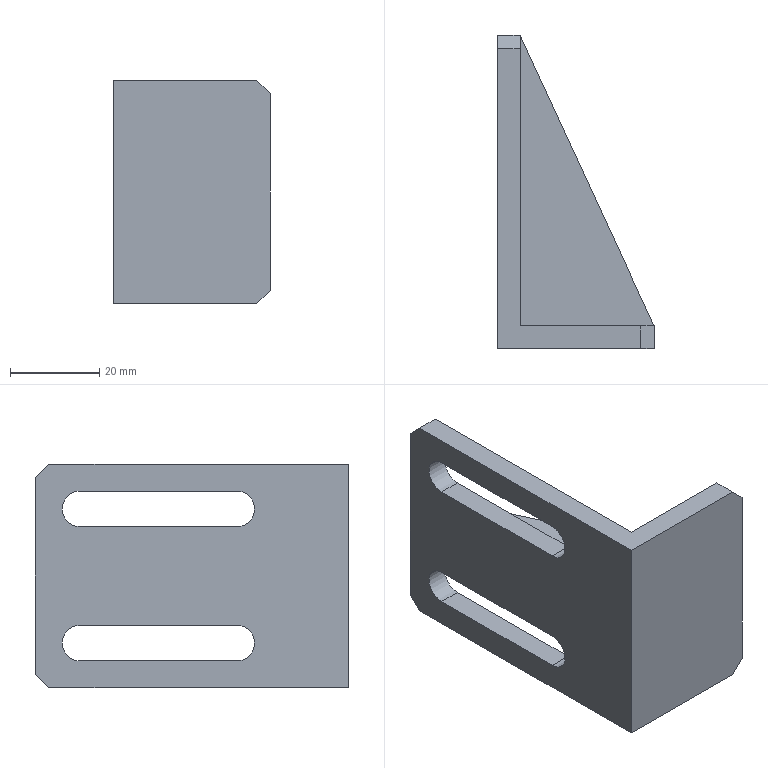Part | STEP file | Guide wheel mechanism revised.sldasm-Part-62 | 1 solid | 25 faces | box 35 x 70 x 50 mm | volume 26482 mm3 | plane 21 | cylinder 4 | commonest cylinder face diameters 8 x4
STEP:
#1=CARTESIAN_POINT('',(35.,5.,-2.5));
#2=VERTEX_POINT('',#1);
#3=CARTESIAN_POINT('',(35.,5.,-22.));
#4=VERTEX_POINT('',#3);
#5=CARTESIAN_POINT('',(35.,5.,25.));
#6=DIRECTION('',(0.,0.,-1.));
#7=VECTOR('',#6,1000.);
#8=LINE('',#5,#7);
#9=EDGE_CURVE('',#2,#4,#8,.T.);
#10=ORIENTED_EDGE('',*,*,#9,.T.);
#11=CARTESIAN_POINT('',(32.,5.,-25.));
#12=VERTEX_POINT('',#11);
#13=CARTESIAN_POINT('',(41.,5.,-16.));
#14=DIRECTION('',(-0.7071,0.,-0.7071));
#15=VECTOR('',#14,1000.);
#16=LINE('',#13,#15);
#17=EDGE_CURVE('',#4,#12,#16,.T.);
#18=ORIENTED_EDGE('',*,*,#17,.T.);
#19=CARTESIAN_POINT('',(5.,5.,-25.));
#20=VERTEX_POINT('',#19);
#21=CARTESIAN_POINT('',(0.,5.,-25.));
#22=DIRECTION('',(1.,0.,0.));
#23=VECTOR('',#22,1000.);
#24=LINE('',#21,#23);
#25=EDGE_CURVE('',#20,#12,#24,.T.);
#26=ORIENTED_EDGE('',*,*,#25,.F.);
#27=CARTESIAN_POINT('',(5.,5.,-2.5));
#28=VERTEX_POINT('',#27);
#29=CARTESIAN_POINT('',(5.,5.,25.));
#30=DIRECTION('',(0.,0.,-1.));
#31=VECTOR('',#30,1000.);
#32=LINE('',#29,#31);
#33=EDGE_CURVE('',#28,#20,#32,.T.);
#34=ORIENTED_EDGE('',*,*,#33,.F.);
#35=CARTESIAN_POINT('',(35.,5.,-2.5));
#36=DIRECTION('',(1.,0.,0.));
#37=VECTOR('',#36,1000.);
#38=LINE('',#35,#37);
#39=EDGE_CURVE('',#28,#2,#38,.T.);
#40=ORIENTED_EDGE('',*,*,#39,.T.);
#41=EDGE_LOOP('',(#10,#18,#26,#34,#40));
#42=FACE_OUTER_BOUND('',#41,.T.);
#43=CARTESIAN_POINT('',(0.,5.,25.));
#44=DIRECTION('',(0.,1.,0.));
#45=DIRECTION('',(0.,0.,1.));
#46=AXIS2_PLACEMENT_3D('',#43,#44,#45);
#47=PLANE('',#46);
#48=ADVANCED_FACE('',(#42),#47,.T.);
#49=CARTESIAN_POINT('',(5.,60.,-19.));
#50=VERTEX_POINT('',#49);
#51=CARTESIAN_POINT('',(5.,60.,-11.));
#52=VERTEX_POINT('',#51);
#53=CARTESIAN_POINT('',(5.,60.,-15.));
#54=DIRECTION('',(1.,0.,0.));
#55=DIRECTION('',(0.,0.,-1.));
#56=AXIS2_PLACEMENT_3D('',#53,#54,#55);
#57=CIRCLE('',#56,4.);
#58=EDGE_CURVE('',#50,#52,#57,.T.);
#59=ORIENTED_EDGE('',*,*,#58,.F.);
#60=CARTESIAN_POINT('',(5.,25.,-19.));
#61=VERTEX_POINT('',#60);
#62=CARTESIAN_POINT('',(5.,60.,-19.));
#63=DIRECTION('',(0.,1.,0.));
#64=VECTOR('',#63,1000.);
#65=LINE('',#62,#64);
#66=EDGE_CURVE('',#61,#50,#65,.T.);
#67=ORIENTED_EDGE('',*,*,#66,.F.);
#68=CARTESIAN_POINT('',(5.,25.,-11.));
#69=VERTEX_POINT('',#68);
#70=CARTESIAN_POINT('',(5.,25.,-15.));
#71=DIRECTION('',(1.,0.,0.));
#72=DIRECTION('',(0.,0.,-1.));
#73=AXIS2_PLACEMENT_3D('',#70,#71,#72);
#74=CIRCLE('',#73,4.);
#75=EDGE_CURVE('',#69,#61,#74,.T.);
#76=ORIENTED_EDGE('',*,*,#75,.F.);
#77=CARTESIAN_POINT('',(5.,60.,-11.));
#78=DIRECTION('',(0.,-1.,0.));
#79=VECTOR('',#78,1000.);
#80=LINE('',#77,#79);
#81=EDGE_CURVE('',#52,#69,#80,.T.);
#82=ORIENTED_EDGE('',*,*,#81,.F.);
#83=EDGE_LOOP('',(#59,#67,#76,#82));
#84=FACE_BOUND('',#83,.T.);
#85=CARTESIAN_POINT('',(5.,67.,-25.));
#86=VERTEX_POINT('',#85);
#87=CARTESIAN_POINT('',(5.,0.,-25.));
#88=DIRECTION('',(0.,-1.,0.));
#89=VECTOR('',#88,1000.);
#90=LINE('',#87,#89);
#91=EDGE_CURVE('',#86,#20,#90,.T.);
#92=ORIENTED_EDGE('',*,*,#91,.F.);
#93=CARTESIAN_POINT('',(5.,70.,-22.));
#94=VERTEX_POINT('',#93);
#95=CARTESIAN_POINT('',(5.,58.5,-33.5));
#96=DIRECTION('',(0.,0.7071,0.7071));
#97=VECTOR('',#96,1000.);
#98=LINE('',#95,#97);
#99=EDGE_CURVE('',#86,#94,#98,.T.);
#100=ORIENTED_EDGE('',*,*,#99,.T.);
#101=CARTESIAN_POINT('',(5.,70.,-2.5));
#102=VERTEX_POINT('',#101);
#103=CARTESIAN_POINT('',(5.,70.,25.));
#104=DIRECTION('',(0.,0.,-1.));
#105=VECTOR('',#104,1000.);
#106=LINE('',#103,#105);
#107=EDGE_CURVE('',#102,#94,#106,.T.);
#108=ORIENTED_EDGE('',*,*,#107,.F.);
#109=CARTESIAN_POINT('',(5.,5.,-2.5));
#110=DIRECTION('',(0.,-1.,0.));
#111=VECTOR('',#110,1000.);
#112=LINE('',#109,#111);
#113=EDGE_CURVE('',#102,#28,#112,.T.);
#114=ORIENTED_EDGE('',*,*,#113,.T.);
#115=ORIENTED_EDGE('',*,*,#33,.T.);
#116=EDGE_LOOP('',(#92,#100,#108,#114,#115));
#117=FACE_OUTER_BOUND('',#116,.T.);
#118=CARTESIAN_POINT('',(5.,0.,25.));
#119=DIRECTION('',(1.,0.,0.));
#120=DIRECTION('',(0.,0.,-1.));
#121=AXIS2_PLACEMENT_3D('',#118,#119,#120);
#122=PLANE('',#121);
#123=ADVANCED_FACE('',(#84,#117),#122,.T.);
#124=CARTESIAN_POINT('',(35.,0.,22.));
#125=VERTEX_POINT('',#124);
#126=CARTESIAN_POINT('',(35.,0.,-22.));
#127=VERTEX_POINT('',#126);
#128=CARTESIAN_POINT('',(35.,0.,25.));
#129=DIRECTION('',(0.,0.,-1.));
#130=VECTOR('',#129,1000.);
#131=LINE('',#128,#130);
#132=EDGE_CURVE('',#125,#127,#131,.T.);
#133=ORIENTED_EDGE('',*,*,#132,.F.);
#134=CARTESIAN_POINT('',(32.,0.,25.));
#135=VERTEX_POINT('',#134);
#136=CARTESIAN_POINT('',(35.,0.,22.));
#137=DIRECTION('',(-0.7071,0.,0.7071));
#138=VECTOR('',#137,1000.);
#139=LINE('',#136,#138);
#140=EDGE_CURVE('',#125,#135,#139,.T.);
#141=ORIENTED_EDGE('',*,*,#140,.T.);
#142=CARTESIAN_POINT('',(0.,0.,25.));
#143=VERTEX_POINT('',#142);
#144=CARTESIAN_POINT('',(0.,0.,25.));
#145=DIRECTION('',(1.,0.,0.));
#146=VECTOR('',#145,1000.);
#147=LINE('',#144,#146);
#148=EDGE_CURVE('',#143,#135,#147,.T.);
#149=ORIENTED_EDGE('',*,*,#148,.F.);
#150=CARTESIAN_POINT('',(0.,0.,-25.));
#151=VERTEX_POINT('',#150);
#152=CARTESIAN_POINT('',(0.,0.,25.));
#153=DIRECTION('',(0.,0.,-1.));
#154=VECTOR('',#153,1000.);
#155=LINE('',#152,#154);
#156=EDGE_CURVE('',#143,#151,#155,.T.);
#157=ORIENTED_EDGE('',*,*,#156,.T.);
#158=CARTESIAN_POINT('',(32.,0.,-25.));
#159=VERTEX_POINT('',#158);
#160=CARTESIAN_POINT('',(0.,0.,-25.));
#161=DIRECTION('',(1.,0.,0.));
#162=VECTOR('',#161,1000.);
#163=LINE('',#160,#162);
#164=EDGE_CURVE('',#151,#159,#163,.T.);
#165=ORIENTED_EDGE('',*,*,#164,.T.);
#166=CARTESIAN_POINT('',(32.,0.,-25.));
#167=DIRECTION('',(0.7071,0.,0.7071));
#168=VECTOR('',#167,1000.);
#169=LINE('',#166,#168);
#170=EDGE_CURVE('',#159,#127,#169,.T.);
#171=ORIENTED_EDGE('',*,*,#170,.T.);
#172=EDGE_LOOP('',(#133,#141,#149,#157,#165,#171));
#173=FACE_OUTER_BOUND('',#172,.T.);
#174=CARTESIAN_POINT('',(0.,0.,25.));
#175=DIRECTION('',(0.,1.,0.));
#176=DIRECTION('',(0.,0.,1.));
#177=AXIS2_PLACEMENT_3D('',#174,#175,#176);
#178=PLANE('',#177);
#179=ADVANCED_FACE('',(#173),#178,.F.);
#180=CARTESIAN_POINT('',(35.,5.,22.));
#181=VERTEX_POINT('',#180);
#182=CARTESIAN_POINT('',(35.,5.,2.5));
#183=VERTEX_POINT('',#182);
#184=CARTESIAN_POINT('',(35.,5.,25.));
#185=DIRECTION('',(0.,0.,-1.));
#186=VECTOR('',#185,1000.);
#187=LINE('',#184,#186);
#188=EDGE_CURVE('',#181,#183,#187,.T.);
#189=ORIENTED_EDGE('',*,*,#188,.F.);
#190=CARTESIAN_POINT('',(35.,0.,22.));
#191=DIRECTION('',(0.,-1.,0.));
#192=VECTOR('',#191,1000.);
#193=LINE('',#190,#192);
#194=EDGE_CURVE('',#181,#125,#193,.T.);
#195=ORIENTED_EDGE('',*,*,#194,.T.);
#196=ORIENTED_EDGE('',*,*,#132,.T.);
#197=CARTESIAN_POINT('',(35.,5.,-22.));
#198=DIRECTION('',(0.,1.,0.));
#199=VECTOR('',#198,1000.);
#200=LINE('',#197,#199);
#201=EDGE_CURVE('',#127,#4,#200,.T.);
#202=ORIENTED_EDGE('',*,*,#201,.T.);
#203=ORIENTED_EDGE('',*,*,#9,.F.);
#204=CARTESIAN_POINT('',(35.,5.,2.5));
#205=DIRECTION('',(0.,0.,-1.));
#206=VECTOR('',#205,1000.);
#207=LINE('',#204,#206);
#208=EDGE_CURVE('',#183,#2,#207,.T.);
#209=ORIENTED_EDGE('',*,*,#208,.F.);
#210=EDGE_LOOP('',(#189,#195,#196,#202,#203,#209));
#211=FACE_OUTER_BOUND('',#210,.T.);
#212=CARTESIAN_POINT('',(35.,5.,25.));
#213=DIRECTION('',(1.,0.,0.));
#214=DIRECTION('',(0.,0.,-1.));
#215=AXIS2_PLACEMENT_3D('',#212,#213,#214);
#216=PLANE('',#215);
#217=ADVANCED_FACE('',(#211),#216,.T.);
#218=CARTESIAN_POINT('',(5.,5.,25.));
#219=VERTEX_POINT('',#218);
#220=CARTESIAN_POINT('',(32.,5.,25.));
#221=VERTEX_POINT('',#220);
#222=CARTESIAN_POINT('',(0.,5.,25.));
#223=DIRECTION('',(1.,0.,0.));
#224=VECTOR('',#223,1000.);
#225=LINE('',#222,#224);
#226=EDGE_CURVE('',#219,#221,#225,.T.);
#227=ORIENTED_EDGE('',*,*,#226,.T.);
#228=CARTESIAN_POINT('',(16.,5.,41.));
#229=DIRECTION('',(0.7071,0.,-0.7071));
#230=VECTOR('',#229,1000.);
#231=LINE('',#228,#230);
#232=EDGE_CURVE('',#221,#181,#231,.T.);
#233=ORIENTED_EDGE('',*,*,#232,.T.);
#234=ORIENTED_EDGE('',*,*,#188,.T.);
#235=CARTESIAN_POINT('',(5.,5.,2.5));
#236=VERTEX_POINT('',#235);
#237=CARTESIAN_POINT('',(35.,5.,2.5));
#238=DIRECTION('',(1.,0.,0.));
#239=VECTOR('',#238,1000.);
#240=LINE('',#237,#239);
#241=EDGE_CURVE('',#236,#183,#240,.T.);
#242=ORIENTED_EDGE('',*,*,#241,.F.);
#243=CARTESIAN_POINT('',(5.,5.,25.));
#244=DIRECTION('',(0.,0.,-1.));
#245=VECTOR('',#244,1000.);
#246=LINE('',#243,#245);
#247=EDGE_CURVE('',#219,#236,#246,.T.);
#248=ORIENTED_EDGE('',*,*,#247,.F.);
#249=EDGE_LOOP('',(#227,#233,#234,#242,#248));
#250=FACE_OUTER_BOUND('',#249,.T.);
#251=CARTESIAN_POINT('',(0.,5.,25.));
#252=DIRECTION('',(0.,1.,0.));
#253=DIRECTION('',(0.,0.,1.));
#254=AXIS2_PLACEMENT_3D('',#251,#252,#253);
#255=PLANE('',#254);
#256=ADVANCED_FACE('',(#250),#255,.T.);
#257=CARTESIAN_POINT('',(5.,60.,11.));
#258=VERTEX_POINT('',#257);
#259=CARTESIAN_POINT('',(5.,60.,19.));
#260=VERTEX_POINT('',#259);
#261=CARTESIAN_POINT('',(5.,60.,15.));
#262=DIRECTION('',(1.,0.,0.));
#263=DIRECTION('',(0.,0.,-1.));
#264=AXIS2_PLACEMENT_3D('',#261,#262,#263);
#265=CIRCLE('',#264,4.);
#266=EDGE_CURVE('',#258,#260,#265,.T.);
#267=ORIENTED_EDGE('',*,*,#266,.F.);
#268=CARTESIAN_POINT('',(5.,25.,11.));
#269=VERTEX_POINT('',#268);
#270=CARTESIAN_POINT('',(5.,60.,11.));
#271=DIRECTION('',(0.,1.,0.));
#272=VECTOR('',#271,1000.);
#273=LINE('',#270,#272);
#274=EDGE_CURVE('',#269,#258,#273,.T.);
#275=ORIENTED_EDGE('',*,*,#274,.F.);
#276=CARTESIAN_POINT('',(5.,25.,19.));
#277=VERTEX_POINT('',#276);
#278=CARTESIAN_POINT('',(5.,25.,15.));
#279=DIRECTION('',(1.,0.,0.));
#280=DIRECTION('',(0.,0.,-1.));
#281=AXIS2_PLACEMENT_3D('',#278,#279,#280);
#282=CIRCLE('',#281,4.);
#283=EDGE_CURVE('',#277,#269,#282,.T.);
#284=ORIENTED_EDGE('',*,*,#283,.F.);
#285=CARTESIAN_POINT('',(5.,60.,19.));
#286=DIRECTION('',(0.,-1.,0.));
#287=VECTOR('',#286,1000.);
#288=LINE('',#285,#287);
#289=EDGE_CURVE('',#260,#277,#288,.T.);
#290=ORIENTED_EDGE('',*,*,#289,.F.);
#291=EDGE_LOOP('',(#267,#275,#284,#290));
#292=FACE_BOUND('',#291,.T.);
#293=CARTESIAN_POINT('',(5.,70.,22.));
#294=VERTEX_POINT('',#293);
#295=CARTESIAN_POINT('',(5.,70.,2.5));
#296=VERTEX_POINT('',#295);
#297=CARTESIAN_POINT('',(5.,70.,25.));
#298=DIRECTION('',(0.,0.,-1.));
#299=VECTOR('',#298,1000.);
#300=LINE('',#297,#299);
#301=EDGE_CURVE('',#294,#296,#300,.T.);
#302=ORIENTED_EDGE('',*,*,#301,.F.);
#303=CARTESIAN_POINT('',(5.,67.,25.));
#304=VERTEX_POINT('',#303);
#305=CARTESIAN_POINT('',(5.,33.5,58.5));
#306=DIRECTION('',(0.,-0.7071,0.7071));
#307=VECTOR('',#306,1000.);
#308=LINE('',#305,#307);
#309=EDGE_CURVE('',#294,#304,#308,.T.);
#310=ORIENTED_EDGE('',*,*,#309,.T.);
#311=CARTESIAN_POINT('',(5.,0.,25.));
#312=DIRECTION('',(0.,-1.,0.));
#313=VECTOR('',#312,1000.);
#314=LINE('',#311,#313);
#315=EDGE_CURVE('',#304,#219,#314,.T.);
#316=ORIENTED_EDGE('',*,*,#315,.T.);
#317=ORIENTED_EDGE('',*,*,#247,.T.);
#318=CARTESIAN_POINT('',(5.,5.,2.5));
#319=DIRECTION('',(0.,-1.,0.));
#320=VECTOR('',#319,1000.);
#321=LINE('',#318,#320);
#322=EDGE_CURVE('',#296,#236,#321,.T.);
#323=ORIENTED_EDGE('',*,*,#322,.F.);
#324=EDGE_LOOP('',(#302,#310,#316,#317,#323));
#325=FACE_OUTER_BOUND('',#324,.T.);
#326=CARTESIAN_POINT('',(5.,0.,25.));
#327=DIRECTION('',(1.,0.,0.));
#328=DIRECTION('',(0.,0.,-1.));
#329=AXIS2_PLACEMENT_3D('',#326,#327,#328);
#330=PLANE('',#329);
#331=ADVANCED_FACE('',(#292,#325),#330,.T.);
#332=ORIENTED_EDGE('',*,*,#107,.T.);
#333=CARTESIAN_POINT('',(0.,70.,-22.));
#334=VERTEX_POINT('',#333);
#335=CARTESIAN_POINT('',(0.,70.,-22.));
#336=DIRECTION('',(-1.,0.,0.));
#337=VECTOR('',#336,1000.);
#338=LINE('',#335,#337);
#339=EDGE_CURVE('',#94,#334,#338,.T.);
#340=ORIENTED_EDGE('',*,*,#339,.T.);
#341=CARTESIAN_POINT('',(0.,70.,22.));
#342=VERTEX_POINT('',#341);
#343=CARTESIAN_POINT('',(0.,70.,25.));
#344=DIRECTION('',(0.,0.,-1.));
#345=VECTOR('',#344,1000.);
#346=LINE('',#343,#345);
#347=EDGE_CURVE('',#342,#334,#346,.T.);
#348=ORIENTED_EDGE('',*,*,#347,.F.);
#349=CARTESIAN_POINT('',(5.,70.,22.));
#350=DIRECTION('',(1.,0.,0.));
#351=VECTOR('',#350,1000.);
#352=LINE('',#349,#351);
#353=EDGE_CURVE('',#342,#294,#352,.T.);
#354=ORIENTED_EDGE('',*,*,#353,.T.);
#355=ORIENTED_EDGE('',*,*,#301,.T.);
#356=CARTESIAN_POINT('',(5.,70.,2.5));
#357=DIRECTION('',(0.,0.,-1.));
#358=VECTOR('',#357,1000.);
#359=LINE('',#356,#358);
#360=EDGE_CURVE('',#296,#102,#359,.T.);
#361=ORIENTED_EDGE('',*,*,#360,.T.);
#362=EDGE_LOOP('',(#332,#340,#348,#354,#355,#361));
#363=FACE_OUTER_BOUND('',#362,.T.);
#364=CARTESIAN_POINT('',(0.,70.,25.));
#365=DIRECTION('',(0.,1.,0.));
#366=DIRECTION('',(0.,0.,1.));
#367=AXIS2_PLACEMENT_3D('',#364,#365,#366);
#368=PLANE('',#367);
#369=ADVANCED_FACE('',(#363),#368,.T.);
#370=CARTESIAN_POINT('',(0.,25.,-19.));
#371=VERTEX_POINT('',#370);
#372=CARTESIAN_POINT('',(0.,60.,-19.));
#373=VERTEX_POINT('',#372);
#374=CARTESIAN_POINT('',(0.,60.,-19.));
#375=DIRECTION('',(0.,1.,0.));
#376=VECTOR('',#375,1000.);
#377=LINE('',#374,#376);
#378=EDGE_CURVE('',#371,#373,#377,.T.);
#379=ORIENTED_EDGE('',*,*,#378,.T.);
#380=CARTESIAN_POINT('',(0.,60.,-11.));
#381=VERTEX_POINT('',#380);
#382=CARTESIAN_POINT('',(0.,60.,-15.));
#383=DIRECTION('',(1.,0.,0.));
#384=DIRECTION('',(0.,0.,-1.));
#385=AXIS2_PLACEMENT_3D('',#382,#383,#384);
#386=CIRCLE('',#385,4.);
#387=EDGE_CURVE('',#373,#381,#386,.T.);
#388=ORIENTED_EDGE('',*,*,#387,.T.);
#389=CARTESIAN_POINT('',(0.,25.,-11.));
#390=VERTEX_POINT('',#389);
#391=CARTESIAN_POINT('',(0.,60.,-11.));
#392=DIRECTION('',(0.,-1.,0.));
#393=VECTOR('',#392,1000.);
#394=LINE('',#391,#393);
#395=EDGE_CURVE('',#381,#390,#394,.T.);
#396=ORIENTED_EDGE('',*,*,#395,.T.);
#397=CARTESIAN_POINT('',(0.,25.,-15.));
#398=DIRECTION('',(1.,0.,0.));
#399=DIRECTION('',(0.,0.,-1.));
#400=AXIS2_PLACEMENT_3D('',#397,#398,#399);
#401=CIRCLE('',#400,4.);
#402=EDGE_CURVE('',#390,#371,#401,.T.);
#403=ORIENTED_EDGE('',*,*,#402,.T.);
#404=EDGE_LOOP('',(#379,#388,#396,#403));
#405=FACE_BOUND('',#404,.T.);
#406=CARTESIAN_POINT('',(0.,25.,11.));
#407=VERTEX_POINT('',#406);
#408=CARTESIAN_POINT('',(0.,60.,11.));
#409=VERTEX_POINT('',#408);
#410=CARTESIAN_POINT('',(0.,60.,11.));
#411=DIRECTION('',(0.,1.,0.));
#412=VECTOR('',#411,1000.);
#413=LINE('',#410,#412);
#414=EDGE_CURVE('',#407,#409,#413,.T.);
#415=ORIENTED_EDGE('',*,*,#414,.T.);
#416=CARTESIAN_POINT('',(0.,60.,19.));
#417=VERTEX_POINT('',#416);
#418=CARTESIAN_POINT('',(0.,60.,15.));
#419=DIRECTION('',(1.,0.,0.));
#420=DIRECTION('',(0.,0.,-1.));
#421=AXIS2_PLACEMENT_3D('',#418,#419,#420);
#422=CIRCLE('',#421,4.);
#423=EDGE_CURVE('',#409,#417,#422,.T.);
#424=ORIENTED_EDGE('',*,*,#423,.T.);
#425=CARTESIAN_POINT('',(0.,25.,19.));
#426=VERTEX_POINT('',#425);
#427=CARTESIAN_POINT('',(0.,60.,19.));
#428=DIRECTION('',(0.,-1.,0.));
#429=VECTOR('',#428,1000.);
#430=LINE('',#427,#429);
#431=EDGE_CURVE('',#417,#426,#430,.T.);
#432=ORIENTED_EDGE('',*,*,#431,.T.);
#433=CARTESIAN_POINT('',(0.,25.,15.));
#434=DIRECTION('',(1.,0.,0.));
#435=DIRECTION('',(0.,0.,-1.));
#436=AXIS2_PLACEMENT_3D('',#433,#434,#435);
#437=CIRCLE('',#436,4.);
#438=EDGE_CURVE('',#426,#407,#437,.T.);
#439=ORIENTED_EDGE('',*,*,#438,.T.);
#440=EDGE_LOOP('',(#415,#424,#432,#439));
#441=FACE_BOUND('',#440,.T.);
#442=ORIENTED_EDGE('',*,*,#347,.T.);
#443=CARTESIAN_POINT('',(0.,67.,-25.));
#444=VERTEX_POINT('',#443);
#445=CARTESIAN_POINT('',(0.,67.,-25.));
#446=DIRECTION('',(0.,-0.7071,-0.7071));
#447=VECTOR('',#446,1000.);
#448=LINE('',#445,#447);
#449=EDGE_CURVE('',#334,#444,#448,.T.);
#450=ORIENTED_EDGE('',*,*,#449,.T.);
#451=CARTESIAN_POINT('',(0.,0.,-25.));
#452=DIRECTION('',(0.,-1.,0.));
#453=VECTOR('',#452,1000.);
#454=LINE('',#451,#453);
#455=EDGE_CURVE('',#444,#151,#454,.T.);
#456=ORIENTED_EDGE('',*,*,#455,.T.);
#457=ORIENTED_EDGE('',*,*,#156,.F.);
#458=CARTESIAN_POINT('',(0.,67.,25.));
#459=VERTEX_POINT('',#458);
#460=CARTESIAN_POINT('',(0.,0.,25.));
#461=DIRECTION('',(0.,-1.,0.));
#462=VECTOR('',#461,1000.);
#463=LINE('',#460,#462);
#464=EDGE_CURVE('',#459,#143,#463,.T.);
#465=ORIENTED_EDGE('',*,*,#464,.F.);
#466=CARTESIAN_POINT('',(0.,70.,22.));
#467=DIRECTION('',(0.,0.7071,-0.7071));
#468=VECTOR('',#467,1000.);
#469=LINE('',#466,#468);
#470=EDGE_CURVE('',#459,#342,#469,.T.);
#471=ORIENTED_EDGE('',*,*,#470,.T.);
#472=EDGE_LOOP('',(#442,#450,#456,#457,#465,#471));
#473=FACE_OUTER_BOUND('',#472,.T.);
#474=CARTESIAN_POINT('',(0.,0.,25.));
#475=DIRECTION('',(1.,0.,0.));
#476=DIRECTION('',(0.,0.,-1.));
#477=AXIS2_PLACEMENT_3D('',#474,#475,#476);
#478=PLANE('',#477);
#479=ADVANCED_FACE('',(#405,#441,#473),#478,.F.);
#480=ORIENTED_EDGE('',*,*,#148,.T.);
#481=CARTESIAN_POINT('',(32.,5.,25.));
#482=DIRECTION('',(0.,1.,0.));
#483=VECTOR('',#482,1000.);
#484=LINE('',#481,#483);
#485=EDGE_CURVE('',#135,#221,#484,.T.);
#486=ORIENTED_EDGE('',*,*,#485,.T.);
#487=ORIENTED_EDGE('',*,*,#226,.F.);
#488=ORIENTED_EDGE('',*,*,#315,.F.);
#489=CARTESIAN_POINT('',(0.,67.,25.));
#490=DIRECTION('',(-1.,0.,0.));
#491=VECTOR('',#490,1000.);
#492=LINE('',#489,#491);
#493=EDGE_CURVE('',#304,#459,#492,.T.);
#494=ORIENTED_EDGE('',*,*,#493,.T.);
#495=ORIENTED_EDGE('',*,*,#464,.T.);
#496=EDGE_LOOP('',(#480,#486,#487,#488,#494,#495));
#497=FACE_OUTER_BOUND('',#496,.T.);
#498=CARTESIAN_POINT('',(0.,0.,25.));
#499=DIRECTION('',(0.,0.,-1.));
#500=DIRECTION('',(-1.,0.,0.));
#501=AXIS2_PLACEMENT_3D('',#498,#499,#500);
#502=PLANE('',#501);
#503=ADVANCED_FACE('',(#497),#502,.F.);
#504=ORIENTED_EDGE('',*,*,#25,.T.);
#505=CARTESIAN_POINT('',(32.,0.,-25.));
#506=DIRECTION('',(0.,-1.,0.));
#507=VECTOR('',#506,1000.);
#508=LINE('',#505,#507);
#509=EDGE_CURVE('',#12,#159,#508,.T.);
#510=ORIENTED_EDGE('',*,*,#509,.T.);
#511=ORIENTED_EDGE('',*,*,#164,.F.);
#512=ORIENTED_EDGE('',*,*,#455,.F.);
#513=CARTESIAN_POINT('',(0.,67.,-25.));
#514=DIRECTION('',(1.,0.,0.));
#515=VECTOR('',#514,1000.);
#516=LINE('',#513,#515);
#517=EDGE_CURVE('',#444,#86,#516,.T.);
#518=ORIENTED_EDGE('',*,*,#517,.T.);
#519=ORIENTED_EDGE('',*,*,#91,.T.);
#520=EDGE_LOOP('',(#504,#510,#511,#512,#518,#519));
#521=FACE_OUTER_BOUND('',#520,.T.);
#522=CARTESIAN_POINT('',(0.,0.,-25.));
#523=DIRECTION('',(0.,0.,-1.));
#524=DIRECTION('',(-1.,0.,0.));
#525=AXIS2_PLACEMENT_3D('',#522,#523,#524);
#526=PLANE('',#525);
#527=ADVANCED_FACE('',(#521),#526,.T.);
#528=CARTESIAN_POINT('',(5.,70.,-2.5));
#529=DIRECTION('',(-0.4191,0.908,0.));
#530=VECTOR('',#529,1000.);
#531=LINE('',#528,#530);
#532=EDGE_CURVE('',#2,#102,#531,.T.);
#533=ORIENTED_EDGE('',*,*,#532,.T.);
#534=ORIENTED_EDGE('',*,*,#360,.F.);
#535=CARTESIAN_POINT('',(5.,70.,2.5));
#536=DIRECTION('',(-0.4191,0.908,0.));
#537=VECTOR('',#536,1000.);
#538=LINE('',#535,#537);
#539=EDGE_CURVE('',#183,#296,#538,.T.);
#540=ORIENTED_EDGE('',*,*,#539,.F.);
#541=ORIENTED_EDGE('',*,*,#208,.T.);
#542=EDGE_LOOP('',(#533,#534,#540,#541));
#543=FACE_OUTER_BOUND('',#542,.T.);
#544=CARTESIAN_POINT('',(5.,70.,2.5));
#545=DIRECTION('',(-0.908,-0.4191,0.));
#546=DIRECTION('',(0.4191,-0.908,0.));
#547=AXIS2_PLACEMENT_3D('',#544,#545,#546);
#548=PLANE('',#547);
#549=ADVANCED_FACE('',(#543),#548,.F.);
#550=ORIENTED_EDGE('',*,*,#322,.T.);
#551=ORIENTED_EDGE('',*,*,#241,.T.);
#552=ORIENTED_EDGE('',*,*,#539,.T.);
#553=EDGE_LOOP('',(#550,#551,#552));
#554=FACE_OUTER_BOUND('',#553,.T.);
#555=CARTESIAN_POINT('',(0.,0.,2.5));
#556=DIRECTION('',(0.,0.,1.));
#557=DIRECTION('',(1.,0.,0.));
#558=AXIS2_PLACEMENT_3D('',#555,#556,#557);
#559=PLANE('',#558);
#560=ADVANCED_FACE('',(#554),#559,.T.);
#561=ORIENTED_EDGE('',*,*,#113,.F.);
#562=ORIENTED_EDGE('',*,*,#532,.F.);
#563=ORIENTED_EDGE('',*,*,#39,.F.);
#564=EDGE_LOOP('',(#561,#562,#563));
#565=FACE_OUTER_BOUND('',#564,.T.);
#566=CARTESIAN_POINT('',(0.,0.,-2.5));
#567=DIRECTION('',(0.,0.,1.));
#568=DIRECTION('',(1.,0.,0.));
#569=AXIS2_PLACEMENT_3D('',#566,#567,#568);
#570=PLANE('',#569);
#571=ADVANCED_FACE('',(#565),#570,.F.);
#572=ORIENTED_EDGE('',*,*,#232,.F.);
#573=ORIENTED_EDGE('',*,*,#485,.F.);
#574=ORIENTED_EDGE('',*,*,#140,.F.);
#575=ORIENTED_EDGE('',*,*,#194,.F.);
#576=EDGE_LOOP('',(#572,#573,#574,#575));
#577=FACE_OUTER_BOUND('',#576,.T.);
#578=CARTESIAN_POINT('',(35.,5.,22.));
#579=DIRECTION('',(0.7071,0.,0.7071));
#580=DIRECTION('',(0.,1.,0.));
#581=AXIS2_PLACEMENT_3D('',#578,#579,#580);
#582=PLANE('',#581);
#583=ADVANCED_FACE('',(#577),#582,.T.);
#584=ORIENTED_EDGE('',*,*,#17,.F.);
#585=ORIENTED_EDGE('',*,*,#201,.F.);
#586=ORIENTED_EDGE('',*,*,#170,.F.);
#587=ORIENTED_EDGE('',*,*,#509,.F.);
#588=EDGE_LOOP('',(#584,#585,#586,#587));
#589=FACE_OUTER_BOUND('',#588,.T.);
#590=CARTESIAN_POINT('',(32.,0.,-25.));
#591=DIRECTION('',(-0.7071,0.,0.7071));
#592=DIRECTION('',(0.,-1.,0.));
#593=AXIS2_PLACEMENT_3D('',#590,#591,#592);
#594=PLANE('',#593);
#595=ADVANCED_FACE('',(#589),#594,.F.);
#596=ORIENTED_EDGE('',*,*,#449,.F.);
#597=ORIENTED_EDGE('',*,*,#339,.F.);
#598=ORIENTED_EDGE('',*,*,#99,.F.);
#599=ORIENTED_EDGE('',*,*,#517,.F.);
#600=EDGE_LOOP('',(#596,#597,#598,#599));
#601=FACE_OUTER_BOUND('',#600,.T.);
#602=CARTESIAN_POINT('',(0.,67.,-25.));
#603=DIRECTION('',(0.,-0.7071,0.7071));
#604=DIRECTION('',(1.,0.,0.));
#605=AXIS2_PLACEMENT_3D('',#602,#603,#604);
#606=PLANE('',#605);
#607=ADVANCED_FACE('',(#601),#606,.F.);
#608=ORIENTED_EDGE('',*,*,#470,.F.);
#609=ORIENTED_EDGE('',*,*,#493,.F.);
#610=ORIENTED_EDGE('',*,*,#309,.F.);
#611=ORIENTED_EDGE('',*,*,#353,.F.);
#612=EDGE_LOOP('',(#608,#609,#610,#611));
#613=FACE_OUTER_BOUND('',#612,.T.);
#614=CARTESIAN_POINT('',(0.,70.,22.));
#615=DIRECTION('',(0.,0.7071,0.7071));
#616=DIRECTION('',(-1.,0.,0.));
#617=AXIS2_PLACEMENT_3D('',#614,#615,#616);
#618=PLANE('',#617);
#619=ADVANCED_FACE('',(#613),#618,.T.);
#620=ORIENTED_EDGE('',*,*,#266,.T.);
#621=CARTESIAN_POINT('',(0.,60.,19.));
#622=DIRECTION('',(1.,0.,0.));
#623=VECTOR('',#622,1000.);
#624=LINE('',#621,#623);
#625=EDGE_CURVE('',#417,#260,#624,.T.);
#626=ORIENTED_EDGE('',*,*,#625,.F.);
#627=ORIENTED_EDGE('',*,*,#423,.F.);
#628=CARTESIAN_POINT('',(0.,60.,11.));
#629=DIRECTION('',(1.,0.,0.));
#630=VECTOR('',#629,1000.);
#631=LINE('',#628,#630);
#632=EDGE_CURVE('',#409,#258,#631,.T.);
#633=ORIENTED_EDGE('',*,*,#632,.T.);
#634=EDGE_LOOP('',(#620,#626,#627,#633));
#635=FACE_OUTER_BOUND('',#634,.T.);
#636=CARTESIAN_POINT('',(0.,60.,15.));
#637=DIRECTION('',(1.,0.,0.));
#638=DIRECTION('',(0.,0.,-1.));
#639=AXIS2_PLACEMENT_3D('',#636,#637,#638);
#640=CYLINDRICAL_SURFACE('',#639,4.);
#641=ADVANCED_FACE('',(#635),#640,.F.);
#642=ORIENTED_EDGE('',*,*,#274,.T.);
#643=ORIENTED_EDGE('',*,*,#632,.F.);
#644=ORIENTED_EDGE('',*,*,#414,.F.);
#645=CARTESIAN_POINT('',(0.,25.,11.));
#646=DIRECTION('',(1.,0.,0.));
#647=VECTOR('',#646,1000.);
#648=LINE('',#645,#647);
#649=EDGE_CURVE('',#407,#269,#648,.T.);
#650=ORIENTED_EDGE('',*,*,#649,.T.);
#651=EDGE_LOOP('',(#642,#643,#644,#650));
#652=FACE_OUTER_BOUND('',#651,.T.);
#653=CARTESIAN_POINT('',(0.,60.,11.));
#654=DIRECTION('',(0.,0.,-1.));
#655=DIRECTION('',(0.,1.,0.));
#656=AXIS2_PLACEMENT_3D('',#653,#654,#655);
#657=PLANE('',#656);
#658=ADVANCED_FACE('',(#652),#657,.F.);
#659=ORIENTED_EDGE('',*,*,#283,.T.);
#660=ORIENTED_EDGE('',*,*,#649,.F.);
#661=ORIENTED_EDGE('',*,*,#438,.F.);
#662=CARTESIAN_POINT('',(0.,25.,19.));
#663=DIRECTION('',(1.,0.,0.));
#664=VECTOR('',#663,1000.);
#665=LINE('',#662,#664);
#666=EDGE_CURVE('',#426,#277,#665,.T.);
#667=ORIENTED_EDGE('',*,*,#666,.T.);
#668=EDGE_LOOP('',(#659,#660,#661,#667));
#669=FACE_OUTER_BOUND('',#668,.T.);
#670=CARTESIAN_POINT('',(0.,25.,15.));
#671=DIRECTION('',(1.,0.,0.));
#672=DIRECTION('',(0.,0.,-1.));
#673=AXIS2_PLACEMENT_3D('',#670,#671,#672);
#674=CYLINDRICAL_SURFACE('',#673,4.);
#675=ADVANCED_FACE('',(#669),#674,.F.);
#676=ORIENTED_EDGE('',*,*,#289,.T.);
#677=ORIENTED_EDGE('',*,*,#666,.F.);
#678=ORIENTED_EDGE('',*,*,#431,.F.);
#679=ORIENTED_EDGE('',*,*,#625,.T.);
#680=EDGE_LOOP('',(#676,#677,#678,#679));
#681=FACE_OUTER_BOUND('',#680,.T.);
#682=CARTESIAN_POINT('',(0.,60.,19.));
#683=DIRECTION('',(0.,0.,1.));
#684=DIRECTION('',(0.,-1.,0.));
#685=AXIS2_PLACEMENT_3D('',#682,#683,#684);
#686=PLANE('',#685);
#687=ADVANCED_FACE('',(#681),#686,.F.);
#688=ORIENTED_EDGE('',*,*,#58,.T.);
#689=CARTESIAN_POINT('',(0.,60.,-11.));
#690=DIRECTION('',(1.,0.,0.));
#691=VECTOR('',#690,1000.);
#692=LINE('',#689,#691);
#693=EDGE_CURVE('',#381,#52,#692,.T.);
#694=ORIENTED_EDGE('',*,*,#693,.F.);
#695=ORIENTED_EDGE('',*,*,#387,.F.);
#696=CARTESIAN_POINT('',(0.,60.,-19.));
#697=DIRECTION('',(1.,0.,0.));
#698=VECTOR('',#697,1000.);
#699=LINE('',#696,#698);
#700=EDGE_CURVE('',#373,#50,#699,.T.);
#701=ORIENTED_EDGE('',*,*,#700,.T.);
#702=EDGE_LOOP('',(#688,#694,#695,#701));
#703=FACE_OUTER_BOUND('',#702,.T.);
#704=CARTESIAN_POINT('',(0.,60.,-15.));
#705=DIRECTION('',(1.,0.,0.));
#706=DIRECTION('',(0.,0.,-1.));
#707=AXIS2_PLACEMENT_3D('',#704,#705,#706);
#708=CYLINDRICAL_SURFACE('',#707,4.);
#709=ADVANCED_FACE('',(#703),#708,.F.);
#710=ORIENTED_EDGE('',*,*,#66,.T.);
#711=ORIENTED_EDGE('',*,*,#700,.F.);
#712=ORIENTED_EDGE('',*,*,#378,.F.);
#713=CARTESIAN_POINT('',(0.,25.,-19.));
#714=DIRECTION('',(1.,0.,0.));
#715=VECTOR('',#714,1000.);
#716=LINE('',#713,#715);
#717=EDGE_CURVE('',#371,#61,#716,.T.);
#718=ORIENTED_EDGE('',*,*,#717,.T.);
#719=EDGE_LOOP('',(#710,#711,#712,#718));
#720=FACE_OUTER_BOUND('',#719,.T.);
#721=CARTESIAN_POINT('',(0.,60.,-19.));
#722=DIRECTION('',(0.,0.,-1.));
#723=DIRECTION('',(-1.,0.,0.));
#724=AXIS2_PLACEMENT_3D('',#721,#722,#723);
#725=PLANE('',#724);
#726=ADVANCED_FACE('',(#720),#725,.F.);
#727=ORIENTED_EDGE('',*,*,#75,.T.);
#728=ORIENTED_EDGE('',*,*,#717,.F.);
#729=ORIENTED_EDGE('',*,*,#402,.F.);
#730=CARTESIAN_POINT('',(0.,25.,-11.));
#731=DIRECTION('',(1.,0.,0.));
#732=VECTOR('',#731,1000.);
#733=LINE('',#730,#732);
#734=EDGE_CURVE('',#390,#69,#733,.T.);
#735=ORIENTED_EDGE('',*,*,#734,.T.);
#736=EDGE_LOOP('',(#727,#728,#729,#735));
#737=FACE_OUTER_BOUND('',#736,.T.);
#738=CARTESIAN_POINT('',(0.,25.,-15.));
#739=DIRECTION('',(1.,0.,0.));
#740=DIRECTION('',(0.,0.,-1.));
#741=AXIS2_PLACEMENT_3D('',#738,#739,#740);
#742=CYLINDRICAL_SURFACE('',#741,4.);
#743=ADVANCED_FACE('',(#737),#742,.F.);
#744=ORIENTED_EDGE('',*,*,#81,.T.);
#745=ORIENTED_EDGE('',*,*,#734,.F.);
#746=ORIENTED_EDGE('',*,*,#395,.F.);
#747=ORIENTED_EDGE('',*,*,#693,.T.);
#748=EDGE_LOOP('',(#744,#745,#746,#747));
#749=FACE_OUTER_BOUND('',#748,.T.);
#750=CARTESIAN_POINT('',(0.,60.,-11.));
#751=DIRECTION('',(0.,0.,1.));
#752=DIRECTION('',(0.,-1.,0.));
#753=AXIS2_PLACEMENT_3D('',#750,#751,#752);
#754=PLANE('',#753);
#755=ADVANCED_FACE('',(#749),#754,.F.);
#756=CLOSED_SHELL('',(#48,#123,#179,#217,#256,#331,#369,#479,#503,#527,#549,#560,#571,#583,#595,#607,#619,#641,#658,#675,#687,#709,#726,#743,#755));
#757=MANIFOLD_SOLID_BREP('',#756);
#758=CARTESIAN_POINT('',(0.,0.,0.));
#759=DIRECTION('',(0.,0.,1.));
#760=DIRECTION('',(1.,0.,0.));
#761=AXIS2_PLACEMENT_3D('',#758,#759,#760);
#762=(LENGTH_UNIT()NAMED_UNIT(*)SI_UNIT(.MILLI.,.METRE.));
#763=UNCERTAINTY_MEASURE_WITH_UNIT(LENGTH_MEASURE(0.00001),#762,'','');
#764=(NAMED_UNIT(*)PLANE_ANGLE_UNIT()SI_UNIT($,.RADIAN.));
#765=(NAMED_UNIT(*)SI_UNIT($,.STERADIAN.)SOLID_ANGLE_UNIT());
#766=(GEOMETRIC_REPRESENTATION_CONTEXT(3)GLOBAL_UNCERTAINTY_ASSIGNED_CONTEXT((#763))GLOBAL_UNIT_ASSIGNED_CONTEXT((#762,#764,#765))REPRESENTATION_CONTEXT('',''));
#767=ADVANCED_BREP_SHAPE_REPRESENTATION('',(#757,#761),#766);